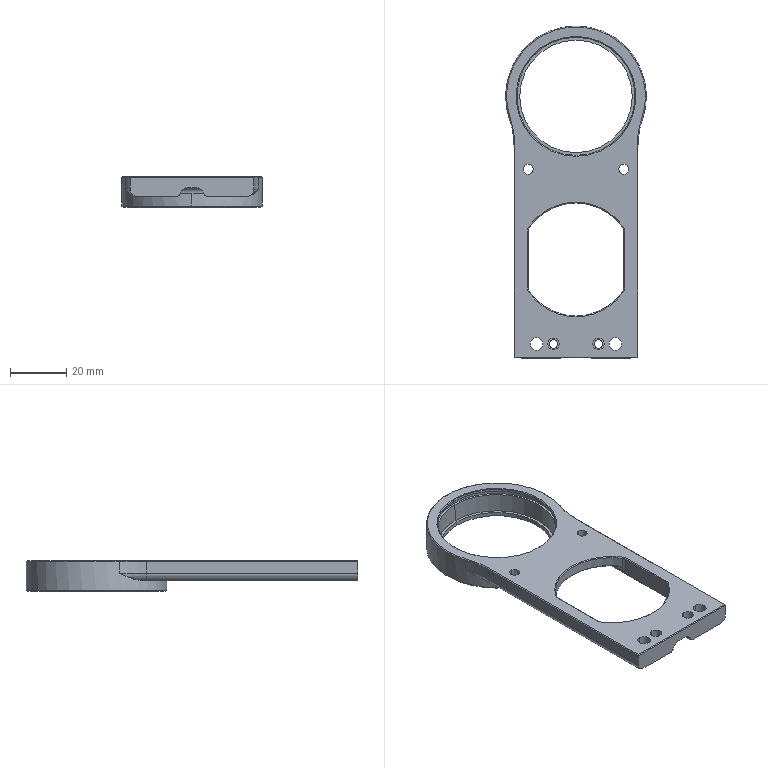NC program | NX | posted with a generic post | part box 50 x 118 x 11 mm
Whole program:
N10 G17 G21 G94 G90
(PLANAR_MILL_1 , TOOL : D6A45)
N12 T01 M6
N14 M5
(ZLEVEL_PROFILE_COPY_1 , TOOL : D10)
N16 T15 M6
N18 G54
N20 G17 G0 G90 X25.439 Y11.571 S9500 M3
N22 G43 Z-41. H15
N24 Z-12.2
N26 G94 G1 X25.868 Y11.9 Z-12.172 F1000.
N28 X44.132 Z-11.214
N30 X44.885 Y11.322 Z-11.165
N32 X46.664 Y9.479 Z-11.031
N34 X48.104 Y7.361 Z-10.896
N36 X49.163 Y5.03 Z-10.762
N38 X49.812 Y2.552 Z-10.628
N40 X50.03 Y0. Z-10.494
N42 X49.812 Y-2.552 Z-10.359
N44 X49.163 Y-5.03 Z-10.225
N46 X48.104 Y-7.361 Z-10.091
N48 X46.664 Y-9.479 Z-9.957
N50 X44.885 Y-11.322 Z-9.822
N52 X44.132 Y-11.9 Z-9.773
N54 X25.868 F3500.
N56 G2 X25.868 Y11.9 R15.
N58 G1 X44.132
N60 G2 X44.132 Y-11.9 R15.
N62 G1 X25.868 Z-9.588
N64 X25.669 Y-11.744 Z-9.585
N66 X24.566 Y-10.776 Z-9.57
N68 X23.965 Y-10.16 Z-9.561
N70 X23.401 Y-9.511 Z-9.553
N72 X22.875 Y-8.83 Z-9.544
N74 X22.388 Y-8.121 Z-9.535
N76 X21.943 Y-7.384 Z-9.527
N78 X21.541 Y-6.623 Z-9.518
N80 X21.184 Y-5.841 Z-9.509
N82 X20.872 Y-5.039 Z-9.5
N84 X20.606 Y-4.221 Z-9.492
N86 X20.388 Y-3.388 Z-9.483
N88 X20.217 Y-2.545 Z-9.474
N90 X20.096 Y-1.693 Z-9.466
N92 X20.023 Y-0.836 Z-9.457
N94 X20. Y0.024 Z-9.448
N96 X20.026 Y0.881 Z-9.439
N98 X20.101 Y1.735 Z-9.431
N100 X20.224 Y2.584 Z-9.422
N102 X20.396 Y3.424 Z-9.413
N104 X20.615 Y4.252 Z-9.405
N106 X20.882 Y5.067 Z-9.396
N108 X21.194 Y5.866 Z-9.387
N110 X21.552 Y6.645 Z-9.379
N112 X21.954 Y7.402 Z-9.37
N114 X22.398 Y8.136 Z-9.361
N116 X22.883 Y8.842 Z-9.353
N118 X23.408 Y9.52 Z-9.344
N120 X23.971 Y10.167 Z-9.335
N122 X24.57 Y10.781 Z-9.326
N124 X25.714 Y11.78 Z-9.311
N126 X25.868 Y11.9 Z-9.309
N128 X44.132 Z-9.124
N130 X44.355 Y11.726 Z-9.121
N132 X45.514 Y10.698 Z-9.105
N134 X46.147 Y10.037 Z-9.096
N136 X46.739 Y9.337 Z-9.087
N138 X47.287 Y8.603 Z-9.078
N140 X47.79 Y7.837 Z-9.068
N142 X48.244 Y7.042 Z-9.059
N144 X48.65 Y6.22 Z-9.05
N146 X49.004 Y5.375 Z-9.04
N148 X49.306 Y4.51 Z-9.031
N150 X49.554 Y3.629 Z-9.022
N152 X49.749 Y2.733 Z-9.013
N154 X49.888 Y1.828 Z-9.003
N156 X49.972 Y0.916 Z-8.994
N158 X50. Y0. Z-8.985
N160 X49.972 Y-0.916 Z-8.975
N162 X49.888 Y-1.828 Z-8.966
N164 X49.749 Y-2.733 Z-8.957
N166 X49.554 Y-3.629 Z-8.948
N168 X49.306 Y-4.51 Z-8.938
N170 X49.004 Y-5.375 Z-8.929
N172 X48.65 Y-6.22 Z-8.92
N174 X48.244 Y-7.042 Z-8.91
N176 X47.79 Y-7.837 Z-8.901
N178 X47.287 Y-8.603 Z-8.892
N180 X46.739 Y-9.337 Z-8.883
N182 X46.147 Y-10.037 Z-8.873
N184 X45.514 Y-10.698 Z-8.864
N186 X44.838 Y-11.323 Z-8.855
N188 X44.132 Y-11.9 Z-8.845
N190 X25.868 Z-8.66
N192 X25.669 Y-11.744 Z-8.658
N194 X24.566 Y-10.776 Z-8.643
N196 X23.965 Y-10.16 Z-8.634
N198 X23.401 Y-9.511 Z-8.625
N200 X22.875 Y-8.83 Z-8.617
N202 X22.388 Y-8.121 Z-8.608
N204 X21.943 Y-7.384 Z-8.599
N206 X21.541 Y-6.623 Z-8.591
N208 X21.184 Y-5.841 Z-8.582
N210 X20.872 Y-5.039 Z-8.573
N212 X20.606 Y-4.221 Z-8.564
N214 X20.388 Y-3.388 Z-8.556
N216 X20.217 Y-2.545 Z-8.547
N218 X20.096 Y-1.693 Z-8.538
N220 X20.023 Y-0.836 Z-8.53
N222 X20. Y0.024 Z-8.521
N224 X20.026 Y0.881 Z-8.512
N226 X20.101 Y1.735 Z-8.503
N228 X20.224 Y2.584 Z-8.495
N230 X20.396 Y3.424 Z-8.486
N232 X20.615 Y4.252 Z-8.477
N234 X20.882 Y5.067 Z-8.469
N236 X21.194 Y5.866 Z-8.46
N238 X21.552 Y6.645 Z-8.451
N240 X21.954 Y7.402 Z-8.443
N242 X22.398 Y8.136 Z-8.434
N244 X22.883 Y8.842 Z-8.425
N246 X23.408 Y9.52 Z-8.417
N248 X23.971 Y10.167 Z-8.408
N250 X24.57 Y10.781 Z-8.399
N252 X25.714 Y11.78 Z-8.384
N254 X25.868 Y11.9 Z-8.382
N256 X44.132 Z-8.197
N258 X44.355 Y11.726 Z-8.194
N260 X45.514 Y10.698 Z-8.178
N262 X46.147 Y10.037 Z-8.169
N264 X46.739 Y9.337 Z-8.16
N266 X47.287 Y8.603 Z-8.15
N268 X47.79 Y7.837 Z-8.141
N270 X48.244 Y7.042 Z-8.132
N272 X48.65 Y6.22 Z-8.122
N274 X49.004 Y5.375 Z-8.113
N276 X49.306 Y4.51 Z-8.104
N278 X49.554 Y3.629 Z-8.095
N280 X49.749 Y2.733 Z-8.085
N282 X49.888 Y1.828 Z-8.076
N284 X49.972 Y0.916 Z-8.067
N286 X50. Y0. Z-8.057
N288 X49.972 Y-0.916 Z-8.048
N290 X49.888 Y-1.828 Z-8.039
N292 X49.749 Y-2.733 Z-8.03
N294 X49.554 Y-3.629 Z-8.02
N296 X49.306 Y-4.51 Z-8.011
N298 X49.004 Y-5.375 Z-8.002
N300 X48.65 Y-6.22 Z-7.992
N302 X48.244 Y-7.042 Z-7.983
N304 X47.79 Y-7.837 Z-7.974
N306 X47.287 Y-8.603 Z-7.965
N308 X46.739 Y-9.337 Z-7.955
N310 X46.147 Y-10.037 Z-7.946
N312 X45.514 Y-10.698 Z-7.937
N314 X44.841 Y-11.32 Z-7.927
N316 X44.132 Y-11.9 Z-7.918
N318 X25.868 Z-7.733
N320 X25.669 Y-11.744 Z-7.73
N322 X24.566 Y-10.776 Z-7.716
N324 X23.965 Y-10.16 Z-7.707
N326 X23.401 Y-9.511 Z-7.698
N328 X22.875 Y-8.83 Z-7.689
N330 X22.388 Y-8.121 Z-7.681
N332 X21.943 Y-7.384 Z-7.672
N334 X21.541 Y-6.623 Z-7.663
N336 X21.184 Y-5.841 Z-7.655
N338 X20.872 Y-5.039 Z-7.646
N340 X20.606 Y-4.221 Z-7.637
N342 X20.388 Y-3.388 Z-7.628
N344 X20.217 Y-2.545 Z-7.62
N346 X20.096 Y-1.693 Z-7.611
N348 X20.023 Y-0.836 Z-7.602
N350 X20. Y0.024 Z-7.594
N352 X20.026 Y0.881 Z-7.585
N354 X20.101 Y1.735 Z-7.576
N356 X20.224 Y2.584 Z-7.567
N358 X20.396 Y3.424 Z-7.559
N360 X20.615 Y4.252 Z-7.55
N362 X20.882 Y5.067 Z-7.541
N364 X21.194 Y5.866 Z-7.533
N366 X21.552 Y6.645 Z-7.524
N368 X21.954 Y7.402 Z-7.515
N370 X22.398 Y8.136 Z-7.507
N372 X22.883 Y8.842 Z-7.498
N374 X23.408 Y9.52 Z-7.489
N376 X23.971 Y10.167 Z-7.481
N378 X24.57 Y10.781 Z-7.472
N380 X25.714 Y11.78 Z-7.457
N382 X25.868 Y11.9 Z-7.455
N384 X44.132 Z-7.269
N386 X44.355 Y11.726 Z-7.266
N388 X45.514 Y10.698 Z-7.251
N390 X46.147 Y10.037 Z-7.242
N392 X46.739 Y9.337 Z-7.232
N394 X47.287 Y8.603 Z-7.223
N396 X47.79 Y7.837 Z-7.214
N398 X48.244 Y7.042 Z-7.204
N400 X48.65 Y6.22 Z-7.195
N402 X49.004 Y5.375 Z-7.186
N404 X49.306 Y4.51 Z-7.177
N406 X49.554 Y3.629 Z-7.167
N408 X49.749 Y2.733 Z-7.158
N410 X49.888 Y1.828 Z-7.149
N412 X49.972 Y0.916 Z-7.139
N414 X50. Y0. Z-7.13
N416 X49.972 Y-0.916 Z-7.121
N418 X49.888 Y-1.828 Z-7.112
N420 X49.749 Y-2.733 Z-7.102
N422 X49.554 Y-3.629 Z-7.093
N424 X49.306 Y-4.51 Z-7.084
N426 X49.004 Y-5.375 Z-7.074
N428 X48.65 Y-6.22 Z-7.065
N430 X48.244 Y-7.042 Z-7.056
N432 X47.79 Y-7.837 Z-7.047
N434 X47.287 Y-8.603 Z-7.037
N436 X46.739 Y-9.337 Z-7.028
N438 X46.147 Y-10.037 Z-7.019
N440 X45.514 Y-10.698 Z-7.009
N442 X44.841 Y-11.32 Z-7.
N444 X44.132 Y-11.9 Z-6.991
N446 X25.868 Z-6.806
N448 X25.669 Y-11.744 Z-6.803
N450 X24.566 Y-10.776 Z-6.788
N452 X23.965 Y-10.16 Z-6.78
N454 X23.401 Y-9.511 Z-6.771
N456 X22.875 Y-8.83 Z-6.762
N458 X22.388 Y-8.121 Z-6.753
N460 X21.943 Y-7.384 Z-6.745
N462 X21.541 Y-6.623 Z-6.736
N464 X21.184 Y-5.841 Z-6.727
N466 X20.872 Y-5.039 Z-6.719
N468 X20.606 Y-4.221 Z-6.71
N470 X20.388 Y-3.388 Z-6.701
N472 X20.217 Y-2.545 Z-6.692
N474 X20.096 Y-1.693 Z-6.684
N476 X20.023 Y-0.836 Z-6.675
N478 X20. Y0.024 Z-6.666
N480 X20.026 Y0.881 Z-6.658
N482 X20.101 Y1.735 Z-6.649
N484 X20.224 Y2.584 Z-6.64
N486 X20.396 Y3.424 Z-6.632
N488 X20.615 Y4.252 Z-6.623
N490 X20.882 Y5.067 Z-6.614
N492 X21.194 Y5.866 Z-6.605
N494 X21.552 Y6.645 Z-6.597
N496 X21.954 Y7.402 Z-6.588
N498 X22.398 Y8.136 Z-6.579
N500 X22.883 Y8.842 Z-6.571
N502 X23.408 Y9.52 Z-6.562
N504 X23.971 Y10.167 Z-6.553
N506 X24.57 Y10.781 Z-6.545
N508 X25.714 Y11.78 Z-6.529
N510 X25.868 Y11.9 Z-6.527
N512 X44.132 Z-6.342
N514 X44.355 Y11.726 Z-6.339
N516 X45.514 Y10.698 Z-6.324
N518 X46.147 Y10.037 Z-6.314
N520 X46.739 Y9.337 Z-6.305
N522 X47.287 Y8.603 Z-6.296
N524 X47.79 Y7.837 Z-6.286
N526 X48.244 Y7.042 Z-6.277
N528 X48.65 Y6.22 Z-6.268
N530 X49.004 Y5.375 Z-6.259
N532 X49.306 Y4.51 Z-6.249
N534 X49.554 Y3.629 Z-6.24
N536 X49.749 Y2.733 Z-6.231
N538 X49.888 Y1.828 Z-6.221
N540 X49.972 Y0.916 Z-6.212
N542 X50. Y0. Z-6.203
N544 X49.972 Y-0.916 Z-6.194
N546 X49.888 Y-1.828 Z-6.184
N548 X49.749 Y-2.733 Z-6.175
N550 X49.554 Y-3.629 Z-6.166
N552 X49.306 Y-4.51 Z-6.156
N554 X49.004 Y-5.375 Z-6.147
N556 X48.65 Y-6.22 Z-6.138
N558 X48.244 Y-7.042 Z-6.129
N560 X47.79 Y-7.837 Z-6.119
N562 X47.287 Y-8.603 Z-6.11
N564 X46.739 Y-9.337 Z-6.101
N566 X46.147 Y-10.037 Z-6.091
N568 X45.514 Y-10.698 Z-6.082
N570 X44.841 Y-11.32 Z-6.073
N572 X44.132 Y-11.9 Z-6.064
N574 X25.868 Z-5.878
N576 X25.669 Y-11.744 Z-5.876
N578 X24.566 Y-10.776 Z-5.861
N580 X23.965 Y-10.16 Z-5.852
N582 X23.401 Y-9.511 Z-5.844
N584 X22.875 Y-8.83 Z-5.835
N586 X22.388 Y-8.121 Z-5.826
N588 X21.943 Y-7.384 Z-5.817
N590 X21.541 Y-6.623 Z-5.809
N592 X21.184 Y-5.841 Z-5.8
N594 X20.872 Y-5.039 Z-5.791
N596 X20.606 Y-4.221 Z-5.783
N598 X20.388 Y-3.388 Z-5.774
N600 X20.217 Y-2.545 Z-5.765
N602 X20.096 Y-1.693 Z-5.756
N604 X20.023 Y-0.836 Z-5.748
N606 X20. Y0.024 Z-5.739
N608 X20.026 Y0.881 Z-5.73
N610 X20.101 Y1.735 Z-5.722
N612 X20.224 Y2.584 Z-5.713
N614 X20.396 Y3.424 Z-5.704
N616 X20.615 Y4.252 Z-5.696
N618 X20.882 Y5.067 Z-5.687
N620 X21.194 Y5.866 Z-5.678
N622 X21.552 Y6.645 Z-5.669
N624 X21.954 Y7.402 Z-5.661
N626 X22.398 Y8.136 Z-5.652
N628 X22.883 Y8.842 Z-5.643
N630 X23.408 Y9.52 Z-5.635
N632 X23.971 Y10.167 Z-5.626
N634 X24.57 Y10.781 Z-5.617
N636 X25.714 Y11.78 Z-5.602
N638 X25.868 Y11.9 Z-5.6
N640 X44.132 Z-5.415
N642 X44.355 Y11.726 Z-5.412
N644 X45.514 Y10.698 Z-5.396
N646 X46.147 Y10.037 Z-5.387
N648 X46.739 Y9.337 Z-5.378
N650 X47.287 Y8.603 Z-5.368
N652 X47.79 Y7.837 Z-5.359
N654 X48.244 Y7.042 Z-5.35
N656 X48.65 Y6.22 Z-5.341
N658 X49.004 Y5.375 Z-5.331
N660 X49.306 Y4.51 Z-5.322
N662 X49.554 Y3.629 Z-5.313
N664 X49.749 Y2.733 Z-5.303
N666 X49.888 Y1.828 Z-5.294
N668 X49.972 Y0.916 Z-5.285
N670 X50. Y0. Z-5.276
N672 X49.972 Y-0.916 Z-5.266
N674 X49.888 Y-1.828 Z-5.257
N676 X49.749 Y-2.733 Z-5.248
N678 X49.554 Y-3.629 Z-5.238
N680 X49.306 Y-4.51 Z-5.229
N682 X49.004 Y-5.375 Z-5.22
N684 X48.65 Y-6.22 Z-5.211
N686 X48.244 Y-7.042 Z-5.201
N688 X47.79 Y-7.837 Z-5.192
N690 X47.287 Y-8.603 Z-5.183
N692 X46.739 Y-9.337 Z-5.173
N694 X46.147 Y-10.037 Z-5.164
N696 X45.514 Y-10.698 Z-5.155
N698 X44.841 Y-11.32 Z-5.146
N700 X44.132 Y-11.9 Z-5.136
N702 X25.868 Z-4.951
N704 X25.669 Y-11.744 Z-4.949
N706 X24.566 Y-10.776 Z-4.934
N708 X23.965 Y-10.16 Z-4.925
N710 X23.401 Y-9.511 Z-4.916
N712 X22.875 Y-8.83 Z-4.908
N714 X22.388 Y-8.121 Z-4.899
N716 X21.943 Y-7.384 Z-4.89
N718 X21.541 Y-6.623 Z-4.881
N720 X21.184 Y-5.841 Z-4.873
N722 X20.872 Y-5.039 Z-4.864
N724 X20.606 Y-4.221 Z-4.855
N726 X20.388 Y-3.388 Z-4.847
N728 X20.217 Y-2.545 Z-4.838
N730 X20.096 Y-1.693 Z-4.829
N732 X20.023 Y-0.836 Z-4.82
N734 X20. Y0.024 Z-4.812
N736 X20.026 Y0.881 Z-4.803
N738 X20.101 Y1.735 Z-4.794
N740 X20.224 Y2.584 Z-4.786
N742 X20.396 Y3.424 Z-4.777
N744 X20.615 Y4.252 Z-4.768
N746 X20.882 Y5.067 Z-4.76
N748 X21.194 Y5.866 Z-4.751
N750 X21.552 Y6.645 Z-4.742
N752 X21.954 Y7.402 Z-4.734
N754 X22.398 Y8.136 Z-4.725
N756 X22.883 Y8.842 Z-4.716
N758 X23.408 Y9.52 Z-4.707
N760 X23.971 Y10.167 Z-4.699
N762 X24.57 Y10.781 Z-4.69
N764 X25.714 Y11.78 Z-4.675
N766 X25.868 Y11.9 Z-4.673
N768 X44.132 Z-4.488
N770 X44.355 Y11.726 Z-4.485
N772 X45.514 Y10.698 Z-4.469
N774 X46.147 Y10.037 Z-4.46
N776 X46.739 Y9.337 Z-4.45
N778 X47.287 Y8.603 Z-4.441
N780 X47.79 Y7.837 Z-4.432
N782 X48.244 Y7.042 Z-4.423
N784 X48.65 Y6.22 Z-4.413
N786 X49.004 Y5.375 Z-4.404
N788 X49.306 Y4.51 Z-4.395
N790 X49.554 Y3.629 Z-4.385
N792 X49.749 Y2.733 Z-4.376
N794 X49.888 Y1.828 Z-4.367
N796 X49.972 Y0.916 Z-4.358
N798 X50. Y0. Z-4.348
N800 X49.972 Y-0.916 Z-4.339
N802 X49.888 Y-1.828 Z-4.33
N804 X49.749 Y-2.733 Z-4.32
N806 X49.554 Y-3.629 Z-4.311
N808 X49.306 Y-4.51 Z-4.302
N810 X49.004 Y-5.375 Z-4.293
N812 X48.65 Y-6.22 Z-4.283
N814 X48.244 Y-7.042 Z-4.274
N816 X47.79 Y-7.837 Z-4.265
N818 X47.287 Y-8.603 Z-4.256
N820 X46.739 Y-9.337 Z-4.246
N822 X46.147 Y-10.037 Z-4.237
N824 X45.514 Y-10.698 Z-4.228
N826 X44.841 Y-11.32 Z-4.218
N828 X44.132 Y-11.9 Z-4.209
N830 X25.868 Z-4.024
N832 X25.669 Y-11.744 Z-4.021
N834 X24.566 Y-10.776 Z-4.007
N836 X23.965 Y-10.16 Z-3.998
N838 X23.401 Y-9.511 Z-3.989
N840 X22.875 Y-8.83 Z-3.98
N842 X22.388 Y-8.121 Z-3.972
N844 X21.943 Y-7.384 Z-3.963
N846 X21.541 Y-6.623 Z-3.954
N848 X21.184 Y-5.841 Z-3.945
N850 X20.872 Y-5.039 Z-3.937
N852 X20.606 Y-4.221 Z-3.928
N854 X20.388 Y-3.388 Z-3.919
N856 X20.217 Y-2.545 Z-3.911
N858 X20.096 Y-1.693 Z-3.902
N860 X20.023 Y-0.836 Z-3.893
N862 X20. Y0.024 Z-3.884
N864 X20.026 Y0.881 Z-3.876
N866 X20.101 Y1.735 Z-3.867
N868 X20.224 Y2.584 Z-3.858
N870 X20.396 Y3.424 Z-3.85
N872 X20.615 Y4.252 Z-3.841
N874 X20.882 Y5.067 Z-3.832
N876 X21.194 Y5.866 Z-3.824
N878 X21.552 Y6.645 Z-3.815
N880 X21.954 Y7.402 Z-3.806
N882 X22.398 Y8.136 Z-3.798
N884 X22.883 Y8.842 Z-3.789
N886 X23.408 Y9.52 Z-3.78
N888 X23.971 Y10.167 Z-3.772
N890 X24.57 Y10.781 Z-3.763
N892 X25.714 Y11.78 Z-3.747
N894 X25.868 Y11.9 Z-3.745
N896 X44.132 Z-3.56
N898 X44.355 Y11.726 Z-3.557
N900 X45.514 Y10.698 Z-3.542
N902 X46.147 Y10.037 Z-3.532
N904 X46.739 Y9.337 Z-3.523
N906 X47.287 Y8.603 Z-3.514
N908 X47.79 Y7.837 Z-3.505
N910 X48.244 Y7.042 Z-3.495
N912 X48.65 Y6.22 Z-3.486
N914 X49.004 Y5.375 Z-3.477
N916 X49.306 Y4.51 Z-3.467
N918 X49.554 Y3.629 Z-3.458
N920 X49.749 Y2.733 Z-3.449
N922 X49.888 Y1.828 Z-3.44
N924 X49.972 Y0.916 Z-3.43
N926 X50. Y0. Z-3.421
N928 X49.972 Y-0.916 Z-3.412
N930 X49.888 Y-1.828 Z-3.402
N932 X49.749 Y-2.733 Z-3.393
N934 X49.554 Y-3.629 Z-3.384
N936 X49.306 Y-4.51 Z-3.375
N938 X49.004 Y-5.375 Z-3.365
N940 X48.65 Y-6.22 Z-3.356
N942 X48.244 Y-7.042 Z-3.347
N944 X47.79 Y-7.837 Z-3.338
N946 X47.287 Y-8.603 Z-3.328
N948 X46.739 Y-9.337 Z-3.319
N950 X46.147 Y-10.037 Z-3.31
N952 X45.514 Y-10.698 Z-3.3
N954 X44.841 Y-11.32 Z-3.291
N956 X44.132 Y-11.9 Z-3.282
N958 X25.868 Z-3.097
N960 X25.669 Y-11.744 Z-3.094
N962 X24.566 Y-10.776 Z-3.079
N964 X23.965 Y-10.16 Z-3.071
N966 X23.401 Y-9.511 Z-3.062
N968 X22.875 Y-8.83 Z-3.053
N970 X22.388 Y-8.121 Z-3.044
N972 X21.943 Y-7.384 Z-3.036
N974 X21.541 Y-6.623 Z-3.027
N976 X21.184 Y-5.841 Z-3.018
N978 X20.872 Y-5.039 Z-3.009
N980 X20.606 Y-4.221 Z-3.001
N982 X20.388 Y-3.388 Z-2.992
N984 X20.217 Y-2.545 Z-2.983
N986 X20.096 Y-1.693 Z-2.975
N988 X20.023 Y-0.836 Z-2.966
N990 X20. Y0.024 Z-2.957
N992 X20.026 Y0.881 Z-2.948
N994 X20.101 Y1.735 Z-2.94
N996 X20.224 Y2.584 Z-2.931
N998 X20.396 Y3.424 Z-2.922
N1000 X20.615 Y4.252 Z-2.914
N1002 X20.882 Y5.067 Z-2.905
N1004 X21.194 Y5.866 Z-2.896
N1006 X21.552 Y6.645 Z-2.888
N1008 X21.954 Y7.402 Z-2.879
N1010 X22.398 Y8.136 Z-2.87
N1012 X22.883 Y8.842 Z-2.862
N1014 X23.408 Y9.52 Z-2.853
N1016 X23.971 Y10.167 Z-2.844
N1018 X24.57 Y10.781 Z-2.836
N1020 X25.714 Y11.78 Z-2.82
N1022 X25.868 Y11.9 Z-2.818
N1024 X44.132 Z-2.633
N1026 X44.355 Y11.726 Z-2.63
N1028 X45.514 Y10.698 Z-2.614
N1030 X46.147 Y10.037 Z-2.605
N1032 X46.739 Y9.337 Z-2.596
N1034 X47.287 Y8.603 Z-2.587
N1036 X47.79 Y7.837 Z-2.577
N1038 X48.244 Y7.042 Z-2.568
N1040 X48.65 Y6.22 Z-2.559
N1042 X49.004 Y5.375 Z-2.549
N1044 X49.306 Y4.51 Z-2.54
N1046 X49.554 Y3.629 Z-2.531
N1048 X49.749 Y2.733 Z-2.522
N1050 X49.888 Y1.828 Z-2.512
N1052 X49.972 Y0.916 Z-2.503
N1054 X50. Y0. Z-2.494
N1056 X49.972 Y-0.916 Z-2.485
N1058 X49.888 Y-1.828 Z-2.475
N1060 X49.749 Y-2.733 Z-2.466
N1062 X49.554 Y-3.629 Z-2.457
N1064 X49.306 Y-4.51 Z-2.447
N1066 X49.004 Y-5.375 Z-2.438
N1068 X48.65 Y-6.22 Z-2.429
N1070 X48.244 Y-7.042 Z-2.42
N1072 X47.79 Y-7.837 Z-2.41
N1074 X47.287 Y-8.603 Z-2.401
N1076 X46.739 Y-9.337 Z-2.392
N1078 X46.147 Y-10.037 Z-2.382
N1080 X45.514 Y-10.698 Z-2.373
N1082 X44.841 Y-11.32 Z-2.364
N1084 X44.132 Y-11.9 Z-2.355
N1086 X25.868 Z-2.169
N1088 X25.669 Y-11.744 Z-2.167
N1090 X24.566 Y-10.776 Z-2.152
N1092 X23.965 Y-10.16 Z-2.143
N1094 X23.401 Y-9.511 Z-2.135
N1096 X22.875 Y-8.83 Z-2.126
N1098 X22.388 Y-8.121 Z-2.117
N1100 X21.943 Y-7.384 Z-2.108
N1102 X21.541 Y-6.623 Z-2.1
N1104 X21.184 Y-5.841 Z-2.091
N1106 X20.872 Y-5.039 Z-2.082
N1108 X20.606 Y-4.221 Z-2.073
N1110 X20.388 Y-3.388 Z-2.065
N1112 X20.217 Y-2.545 Z-2.056
N1114 X20.096 Y-1.693 Z-2.047
N1116 X20.023 Y-0.836 Z-2.039
N1118 X20. Y0.024 Z-2.03
N1120 X20.026 Y0.881 Z-2.021
N1122 X20.101 Y1.735 Z-2.013
N1124 X20.224 Y2.584 Z-2.004
N1126 X20.396 Y3.424 Z-1.995
N1128 X20.615 Y4.252 Z-1.986
N1130 X20.882 Y5.067 Z-1.978
N1132 X21.194 Y5.866 Z-1.969
N1134 X21.552 Y6.645 Z-1.96
N1136 X21.954 Y7.402 Z-1.952
N1138 X22.398 Y8.136 Z-1.943
N1140 X22.883 Y8.842 Z-1.934
N1142 X23.408 Y9.52 Z-1.926
N1144 X23.971 Y10.167 Z-1.917
N1146 X24.57 Y10.781 Z-1.908
N1148 X25.714 Y11.78 Z-1.893
N1150 X25.868 Y11.9 Z-1.891
N1152 X44.132 Z-1.706
N1154 X44.355 Y11.726 Z-1.703
N1156 X45.514 Y10.698 Z-1.687
N1158 X46.147 Y10.037 Z-1.678
N1160 X46.739 Y9.337 Z-1.669
N1162 X47.287 Y8.603 Z-1.659
N1164 X47.79 Y7.837 Z-1.65
N1166 X48.244 Y7.042 Z-1.641
N1168 X48.65 Y6.22 Z-1.631
N1170 X49.004 Y5.375 Z-1.622
N1172 X49.306 Y4.51 Z-1.613
N1174 X49.554 Y3.629 Z-1.604
N1176 X49.749 Y2.733 Z-1.594
N1178 X49.888 Y1.828 Z-1.585
N1180 X49.972 Y0.916 Z-1.576
N1182 X50. Y0. Z-1.567
N1184 X49.972 Y-0.916 Z-1.557
N1186 X49.888 Y-1.828 Z-1.548
N1188 X49.749 Y-2.733 Z-1.539
N1190 X49.554 Y-3.629 Z-1.529
N1192 X49.306 Y-4.51 Z-1.52
N1194 X49.004 Y-5.375 Z-1.511
N1196 X48.65 Y-6.22 Z-1.502
N1198 X48.244 Y-7.042 Z-1.492
N1200 X47.79 Y-7.837 Z-1.483
N1202 X47.287 Y-8.603 Z-1.474
N1204 X46.739 Y-9.337 Z-1.464
N1206 X46.147 Y-10.037 Z-1.455
N1208 X45.514 Y-10.698 Z-1.446
N1210 X44.841 Y-11.32 Z-1.437
N1212 X44.132 Y-11.9 Z-1.427
N1214 X25.868 Z-1.242
N1216 X25.669 Y-11.744 Z-1.24
N1218 X24.566 Y-10.776 Z-1.225
N1220 X23.965 Y-10.16 Z-1.216
N1222 X23.401 Y-9.511 Z-1.207
N1224 X22.875 Y-8.83 Z-1.199
N1226 X22.388 Y-8.121 Z-1.19
N1228 X21.943 Y-7.384 Z-1.181
N1230 X21.541 Y-6.623 Z-1.172
N1232 X21.184 Y-5.841 Z-1.164
N1234 X20.872 Y-5.039 Z-1.155
N1236 X20.606 Y-4.221 Z-1.146
N1238 X20.388 Y-3.388 Z-1.138
N1240 X20.217 Y-2.545 Z-1.129
N1242 X20.096 Y-1.693 Z-1.12
N1244 X20.023 Y-0.836 Z-1.111
N1246 X20. Y0.024 Z-1.103
N1248 X20.026 Y0.881 Z-1.094
N1250 X20.101 Y1.735 Z-1.085
N1252 X20.224 Y2.584 Z-1.077
N1254 X20.396 Y3.424 Z-1.068
N1256 X20.615 Y4.252 Z-1.059
N1258 X20.882 Y5.067 Z-1.051
N1260 X21.194 Y5.866 Z-1.042
N1262 X21.552 Y6.645 Z-1.033
N1264 X21.954 Y7.402 Z-1.024
N1266 X22.398 Y8.136 Z-1.016
N1268 X22.883 Y8.842 Z-1.007
N1270 X23.408 Y9.52 Z-0.998
N1272 X23.971 Y10.167 Z-0.99
N1274 X24.57 Y10.781 Z-0.981
N1276 X25.714 Y11.78 Z-0.966
N1278 X25.868 Y11.9 Z-0.964
N1280 X44.132 Z-0.778
N1282 X44.355 Y11.726 Z-0.776
N1284 X45.514 Y10.698 Z-0.76
N1286 X46.147 Y10.037 Z-0.751
N1288 X46.739 Y9.337 Z-0.741
N1290 X47.287 Y8.603 Z-0.732
N1292 X47.79 Y7.837 Z-0.723
N1294 X48.244 Y7.042 Z-0.714
N1296 X48.65 Y6.22 Z-0.704
N1298 X49.004 Y5.375 Z-0.695
N1300 X49.306 Y4.51 Z-0.686
N1302 X49.554 Y3.629 Z-0.676
N1304 X49.749 Y2.733 Z-0.667
N1306 X49.888 Y1.828 Z-0.658
N1308 X49.972 Y0.916 Z-0.649
N1310 X50. Y0. Z-0.639
N1312 X49.972 Y-0.916 Z-0.63
N1314 X49.888 Y-1.828 Z-0.621
N1316 X49.749 Y-2.733 Z-0.611
N1318 X49.554 Y-3.629 Z-0.602
N1320 X49.306 Y-4.51 Z-0.593
N1322 X49.004 Y-5.375 Z-0.584
N1324 X48.65 Y-6.22 Z-0.574
N1326 X48.244 Y-7.042 Z-0.565
N1328 X47.79 Y-7.837 Z-0.556
N1330 X47.287 Y-8.603 Z-0.546
N1332 X46.739 Y-9.337 Z-0.537
N1334 X46.147 Y-10.037 Z-0.528
N1336 X45.514 Y-10.698 Z-0.519
N1338 X44.841 Y-11.32 Z-0.509
N1340 X44.132 Y-11.9 Z-0.5
N1342 X25.868
N1344 G2 X25.868 Y11.9 R15.
N1346 G1 X44.132
N1348 G2 X44.132 Y-11.9 R15.
N1350 G1 Z-2.
N1352 G0 Z-41.
N1354 M5
N1356 M2